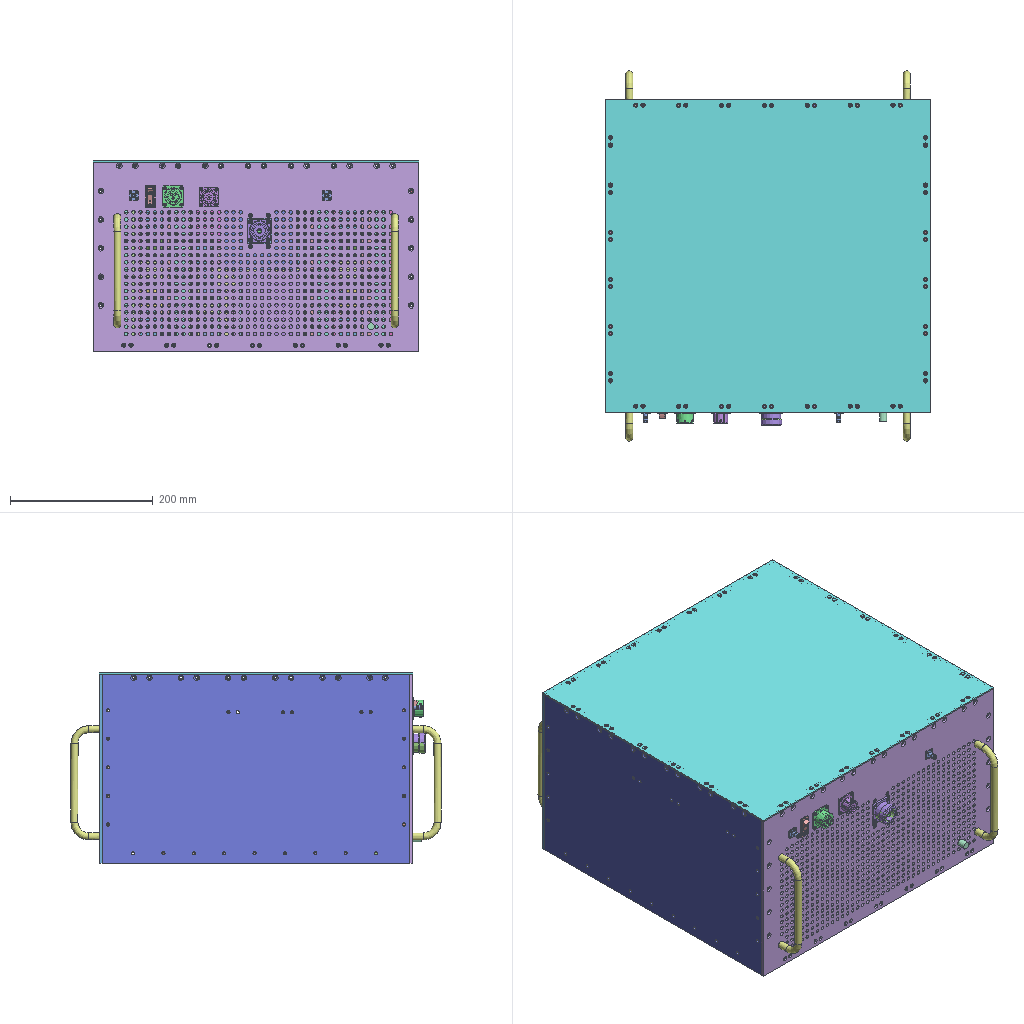Assembly | STEP file | 119 different items | 1042 placed | box 456 x 518 x 267 mm
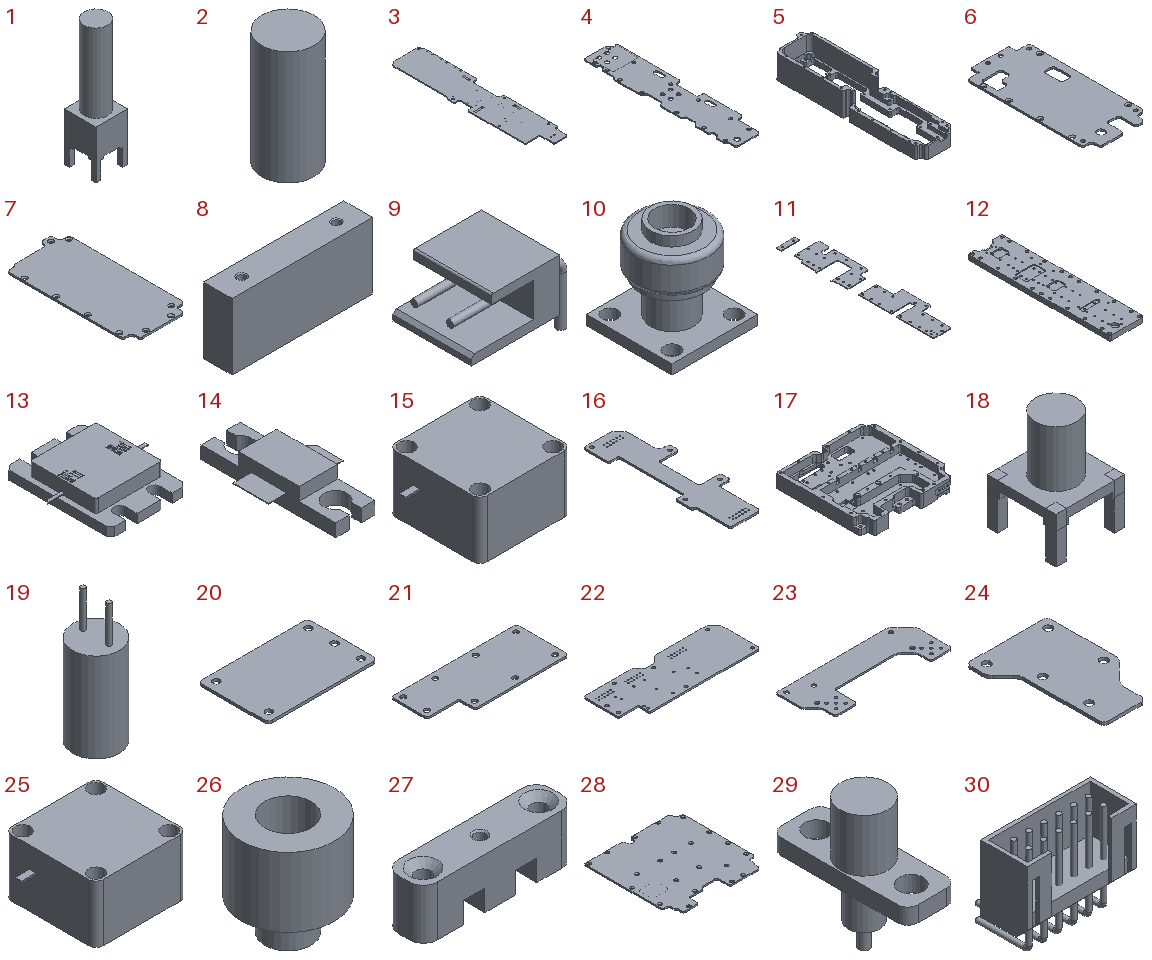Parts list (item | name | quantity | parent item | size | volume):
1 | MCX-KHD20 | x16 | in Final stage amplifier_MODEL | 6 x 6 x 24.3 mm | 456.556 mm3
2 | 1000uf-80V | x64 | in Final stage amplifier control, 48V power filter board_MODEL | 18 x 18 x 39 mm | 9924 mm3
3 | SOLID | x16 | in Final stage amplifier control | 40.98 x 193.1 x 1.2 mm | 8227 mm3
4 | Final stage amplifier cavity inner cover | x16 | in Final stage amplifier_MODEL | 41.47 x 194.01 x 1.5 mm | 9143 mm3
5 | Final stage amplifier cavity | x16 | in Final stage amplifier_MODEL | 49 x 204 x 32.1 mm | 62849 mm3
6 | Final stage amplifier cover 1 | x16 | in Final stage amplifier_MODEL | 49 x 104.5 x 1.5 mm | 6573 mm3
7 | Final stage cover 2 | x16 | in Final stage amplifier_MODEL | 49 x 105.5 x 1.5 mm | 7174 mm3
8 | Final stage amplifier press block | x16 | in Final stage amplifier_MODEL | 29.61 x 6 x 14 mm | 2437 mm3
9 | JL27-02ZJW | x16 | in Final stage amplifier_MODEL | 12.9 x 8.72 x 9.401 mm | 271.213 mm3
10 | N-KFD98 | x32 | in Final stage amplifier_MODEL | 17.5 x 17.5 x 25 mm | 2388 mm3
11 | Final stage amplifier 00 | x16 | in Final stage amplifier_MODEL | 34.739 x 191 x 0.832 mm | 3190 mm3
12 | 53005900 final-stage amplifier red copper | x16 | in Final stage amplifier_MODEL | 49 x 204 x 7 mm | 64981 mm3
13 | GN5359P300V40 | x16 | in Final stage amplifier_MODEL | 23 x 24.1 x 5 mm | 1437 mm3
14 | YP40601625T | x16 | in Final stage amplifier_MODEL | 11.3 x 20.43 x 3.88 mm | 294.314 mm3
15 | UIYDI1212B5300T5900 | x32 | in Final stage amplifier_MODEL | 16.7 x 12.7 x 8 mm | 1173 mm3
16 | 推动功放控制2PCB | x8 | in Driver amplifier module_MODEL | 29.18 x 90.51 x 1.2 mm | 1855 mm3
17 | Driver amplifier module cavity | x8 | in Driver amplifier module_MODEL | 99 x 98 x 14 mm | 63567 mm3
18 | MCX-JHD | x16 | in Driver amplifier module_MODEL | 6 x 6 x 8.9 mm | 97.715 mm3
19 | 118EC225 capacitor | x8 | in Driver amplifier module_MODEL | 6.3 x 6.3 x 17 mm | 376.897 mm3
20 | Driver amplifier PA2PCB | x8 | in Driver amplifier module_MODEL | 34 x 21.66 x 0.832 mm | 597.158 mm3
21 | Driver amplifier PA3PCB | x8 | in Driver amplifier module_MODEL | 52.1 x 21.66 x 0.832 mm | 840 mm3
22 | 推动功放控制1PCB | x8 | in Driver amplifier module_MODEL | 89.69 x 31.78 x 1.2 mm | 3157 mm3
23 | 推动功放1分2PCB | x8 | in Driver amplifier module_MODEL | 66.71 x 26.09 x 0.832 mm | 967.615 mm3
24 | Driver amplifier PA1PCB | x8 | in Driver amplifier module_MODEL | 21.48 x 32.08 x 0.832 mm | 418.678 mm3
25 | UIYDI1212B2800T3400 | x8 | in Driver amplifier module_MODEL | 16.7 x 12.7 x 8 mm | 1173 mm3
26 | Solder post | x32 | in Driver amplifier module_MODEL | 4 x 4 x 4.4 mm | 32.673 mm3
27 | Driver amplifier partition | x16 | in Driver amplifier module_MODEL | 21.48 x 5.5 x 7.1 mm | 643.148 mm3
28 | Driver amplifier module cover | x8 | in Driver amplifier module_MODEL | 99 x 98 x 1.5 mm | 12973 mm3
29 | MCX-KFD1 | x12 | in Driver amplifier module_MODEL, 1 to 8 power divider | 4.7 x 13 x 12.4 mm | 185.301 mm3
30 | JL24-12ZJW | x19 | in Driver amplifier module_MODEL, VSWR protection_MODEL, Control module_MODEL, Front stage module_MODEL | 14.6 x 9.1 x 12.075 mm | 379.843 mm3
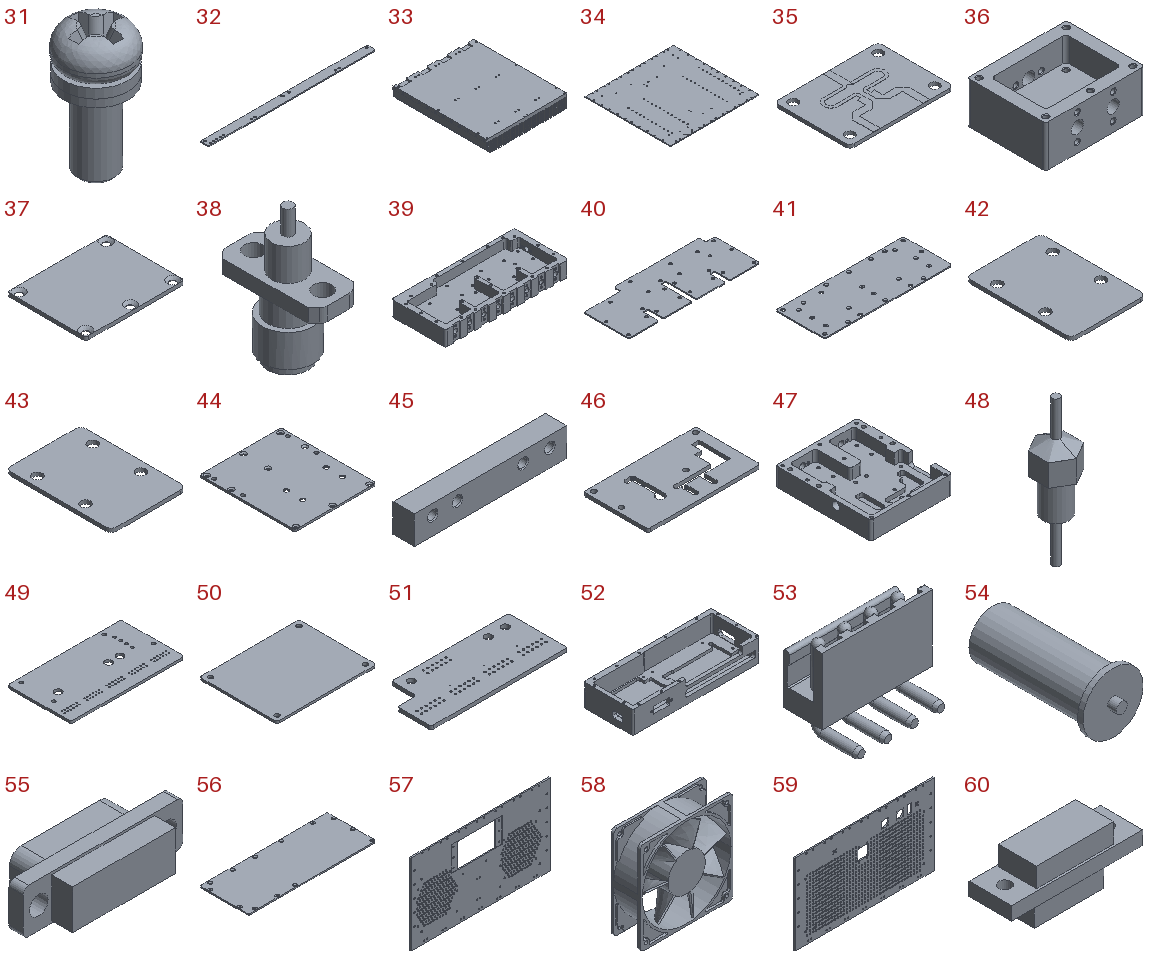31 | Pan head combination screw M2X5 | x8 | in Driver amplifier module_MODEL | 3.5 x 3.5 x 6.7 mm | 32.079 mm3
32 | Power supply board | x4 | in Heat sink | 198 x 10 x 1.2 mm | 2320 mm3
33 | SOLID | x4 | in Heat sink | 200 x 230 x 33.3 mm | 583013 mm3
34 | Chassis bottom plate | x1 | in 27003500整机机箱 | 450 x 430 x 4 mm | 764514 mm3
35 | 1 to 2 power divider PCB | x1 | in 1 to 2 power divider | 25 x 18.18 x 0.832 mm | 351.83 mm3
36 | 1 to 2 power divider cavity | x1 | in 1 to 2 power divider | 33.2 x 26.38 x 14 mm | 8149 mm3
37 | 1 to 2 power divider cover | x1 | in 1 to 2 power divider | 33.2 x 26.38 x 1.2 mm | 1010 mm3
38 | SMA-KFD-4-3 | x14 | in 1 to 2 power divider, 1 to 8 power divider, VSWR protection_MODEL, Frequency synthesizer_MODEL, Front stage module_MODEL | 6.28 x 12.6 x 16.5 mm | 359.204 mm3
39 | 1 to 8 power divider cavity | x1 | in 1 to 8 power divider | 120.8 x 52.94 x 15 mm | 53441 mm3
40 | 1 to 8 power divider PCB | x1 | in 1 to 8 power divider | 110 x 43.34 x 0.832 mm | 3538 mm3
41 | 1 to 8 power divider cover | x1 | in 1 to 8 power divider | 141.709 x 54.52 x 1.2 mm | 9052 mm3
42 | VSWR protection V+PCB | x1 | in VSWR protection_MODEL | 17.08 x 24.07 x 0.832 mm | 328.245 mm3
43 | VSWR protection V-PCB | x1 | in VSWR protection_MODEL | 17.08 x 24.07 x 0.832 mm | 328.245 mm3
44 | VSWR protection cover | x1 | in VSWR protection_MODEL | 60 x 70.12 x 1.5 mm | 6124 mm3
45 | VSWR protection spacer strip | x1 | in VSWR protection_MODEL | 43.08 x 5.97 x 8 mm | 1913 mm3
46 | VSWR protection control PCB | x1 | in VSWR protection_MODEL | 51.4 x 29.58 x 1.6 mm | 2088 mm3
47 | VSWR protection cavity | x1 | in VSWR protection_MODEL | 60 x 70.12 x 13.5 mm | 30547 mm3
48 | Feed through capacitor M3 | x4 | in VSWR protection_MODEL | 4 x 4.619 x 16.5 mm | 73.685 mm3
49 | Control module PCB | x1 | in Control module_MODEL | 76.14 x 42.52 x 1.6 mm | 5007 mm3
50 | Control module MCU PCB | x1 | in Control module_MODEL | 54.57 x 42.52 x 1.2 mm | 2759 mm3
51 | Control module adapter PCB | x1 | in Control module_MODEL | 60.512 x 26.172 x 1.6 mm | 2296 mm3
52 | Control module cavity | x1 | in Control module_MODEL | 141.709 x 54.52 x 25 mm | 59399 mm3
53 | JL27-04ZJW | x1 | in Control module_MODEL | 16.44 x 9.4 x 13.15 mm | 524.314 mm3
54 | Copper solder post M3-11-4.4 | x17 | in Control module_MODEL, 220V main power merge board_MODEL, 48V power filter board_MODEL, 24V input power board_MODEL | 5.5 x 11.8 x 5.5 mm | 131.403 mm3
55 | J30J-21TK | x1 | in Control module_MODEL | 27.4 x 10.9 x 7.6 mm | 1017 mm3
56 | Control module cover | x1 | in Control module_MODEL | 141.709 x 54.52 x 1.5 mm | 11459 mm3
57 | Chassis front panel | x1 | in 27003500整机机箱 | 456 x 4 x 264.7 mm | 404809 mm3
58 | Fan 9WV1224P1H00100 | x2 | in 27003500整机机箱 | 120 x 39.419 x 120 mm | 145446 mm3
59 | Main chassis rear panel | x1 | in 27003500整机机箱 | 456 x 4 x 264.7 mm | 416377 mm3
60 | J30J-15ZKP | x1 | in Frequency synthesizer_MODEL | 23.5 x 7.6 x 10.5 mm | 877.754 mm3
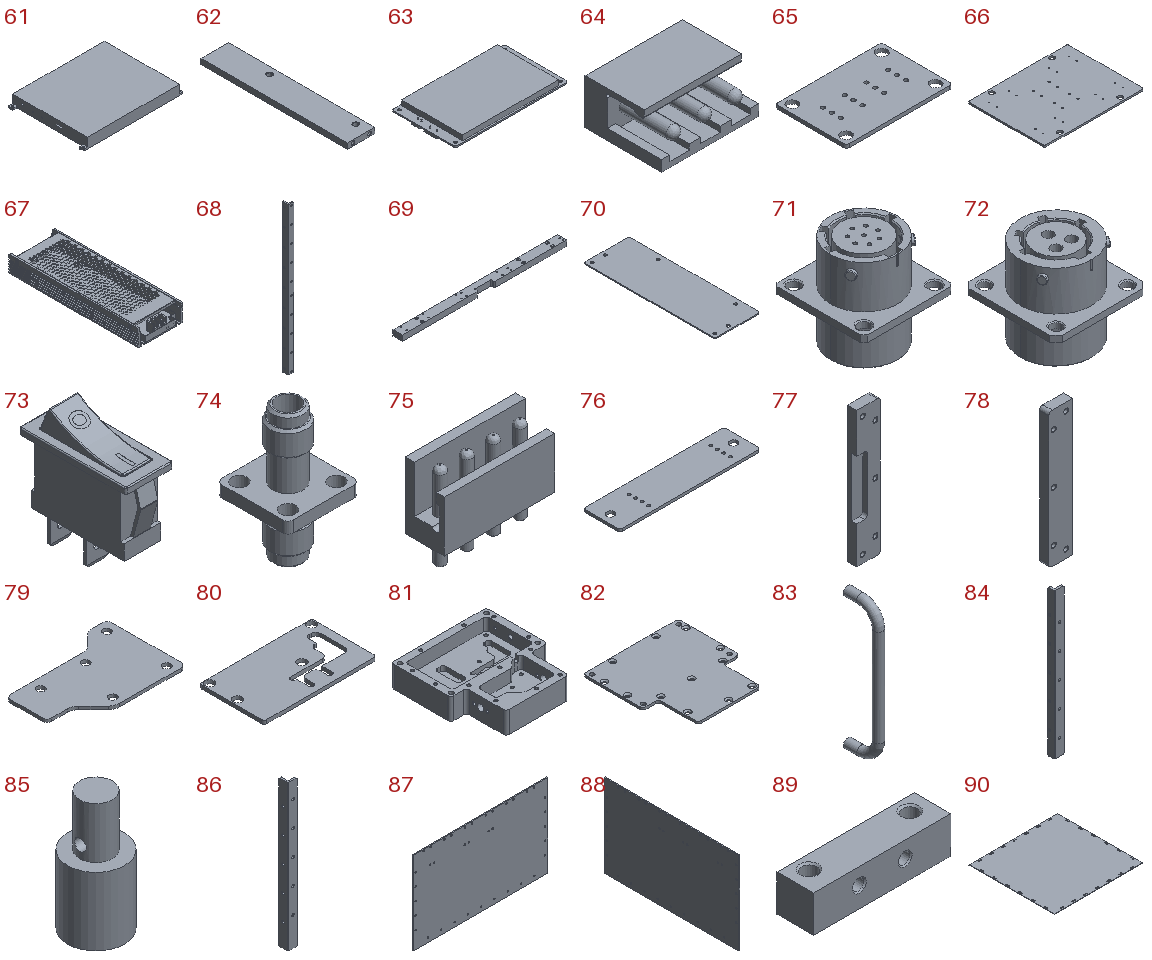61 | SOLID | x1 | in Frequency synthesizer_MODEL | 200 x 150 x 20 mm | 552493 mm3
62 | Power mounting plate | x2 | in 27003500整机机箱 | 20 x 107 x 4 mm | 8429 mm3
63 | Screen OCM800480T500 | x1 | in 27003500整机机箱 | 143.47 x 81 x 10.1 mm | 81087 mm3
64 | JL27-03ZJB | x4 | in 220V main power merge board_MODEL | 12.48 x 11.4 x 5.8 mm | 382.21 mm3
65 | SOLID | x1 | in 220V main power merge board_MODEL | 47.38 x 31.85 x 1.6 mm | 2258 mm3
66 | SOLID | x2 | in 48V power filter board_MODEL | 96.757 x 74.5 x 1.6 mm | 11377 mm3
67 | Power module UHP-500(R) | x1 | in 27003500整机机箱 | 81 x 232 x 31 mm | 117475 mm3
68 | L shaped aluminium angle 1 | x2 | in 27003500整机机箱 | 13 x 15 x 359 mm | 26222 mm3
69 | Chassis spacer strip | x2 | in 27003500整机机箱 | 450 x 25 x 15 mm | 159345 mm3
70 | Mounting block | x1 | in 27003500整机机箱 | 55 x 160 x 1.2 mm | 10487 mm3
71 | Connector Y50X5-1208Z30K | x1 | in 27003500整机机箱 | 27 x 27 x 29.03 mm | 7701 mm3
72 | Connector Y50DX5-1403Z30K | x1 | in 27003500整机机箱 | 30 x 30 x 29.03 mm | 10352 mm3
73 | Rocker switch KCD3-50A | x1 | in 27003500整机机箱 | 13.7 x 31 x 35.877 mm | 6384 mm3
74 | Connector SMA-KKF | x2 | in 27003500整机机箱 | 12.7 x 12.7 x 23.5 mm | 626.237 mm3
75 | JL27-04ZJB | x2 | in 24V input power board_MODEL | 16.44 x 5.8 x 13.5 mm | 568.163 mm3
76 | SOLID | x1 | in 24V input power board_MODEL | 85 x 22 x 1.6 mm | 2905 mm3
77 | Screen mounting block 1 | x1 | in 27003500整机机箱 | 14.18 x 5.5 x 81 mm | 5488 mm3
78 | Screen mounting block 2 | x1 | in 27003500整机机箱 | 14.19 x 5.5 x 81 mm | 6175 mm3
79 | Front stage RF PCB | x1 | in Front stage module_MODEL | 32.08 x 21.48 x 0.832 mm | 418.678 mm3
80 | Front stage control PCB | x1 | in Front stage module_MODEL | 51.4 x 29.58 x 1.6 mm | 2071 mm3
81 | Front stage cavity | x1 | in Front stage module_MODEL | 61.4 x 64.23 x 14 mm | 29019 mm3
82 | Front stage cover | x1 | in Front stage module_MODEL | 61.4 x 64.23 x 1.5 mm | 4977 mm3
83 | SOLID | x8 | in 把手10X150X40-M5 | 10 x 40 x 160 mm | 15544 mm3
84 | L shaped aluminium angle 2 | x1 | in 27003500整机机箱 | 15 x 10.7 x 233 mm | 15474 mm3
85 | Ground post | x1 | in 27003500整机机箱 | 10 x 10 x 21 mm | 1161 mm3
86 | SOLID | x6 | in L shaped aluminium angle 3 | 15 x 15 x 233 mm | 18483 mm3
87 | Chassis left side panel | x1 | in 27003500整机机箱 | 430 x 3 x 264.7 mm | 339377 mm3
88 | Chassis right side panel | x1 | in 27003500整机机箱 | 3 x 430 x 264.7 mm | 339377 mm3
89 | Connector mounting block | x39 | in 27003500整机机箱 | 30 x 8 x 8 mm | 1701 mm3
90 | Chassis cover | x1 | in 27003500整机机箱 | 456 x 438 x 2 mm | 397913 mm3
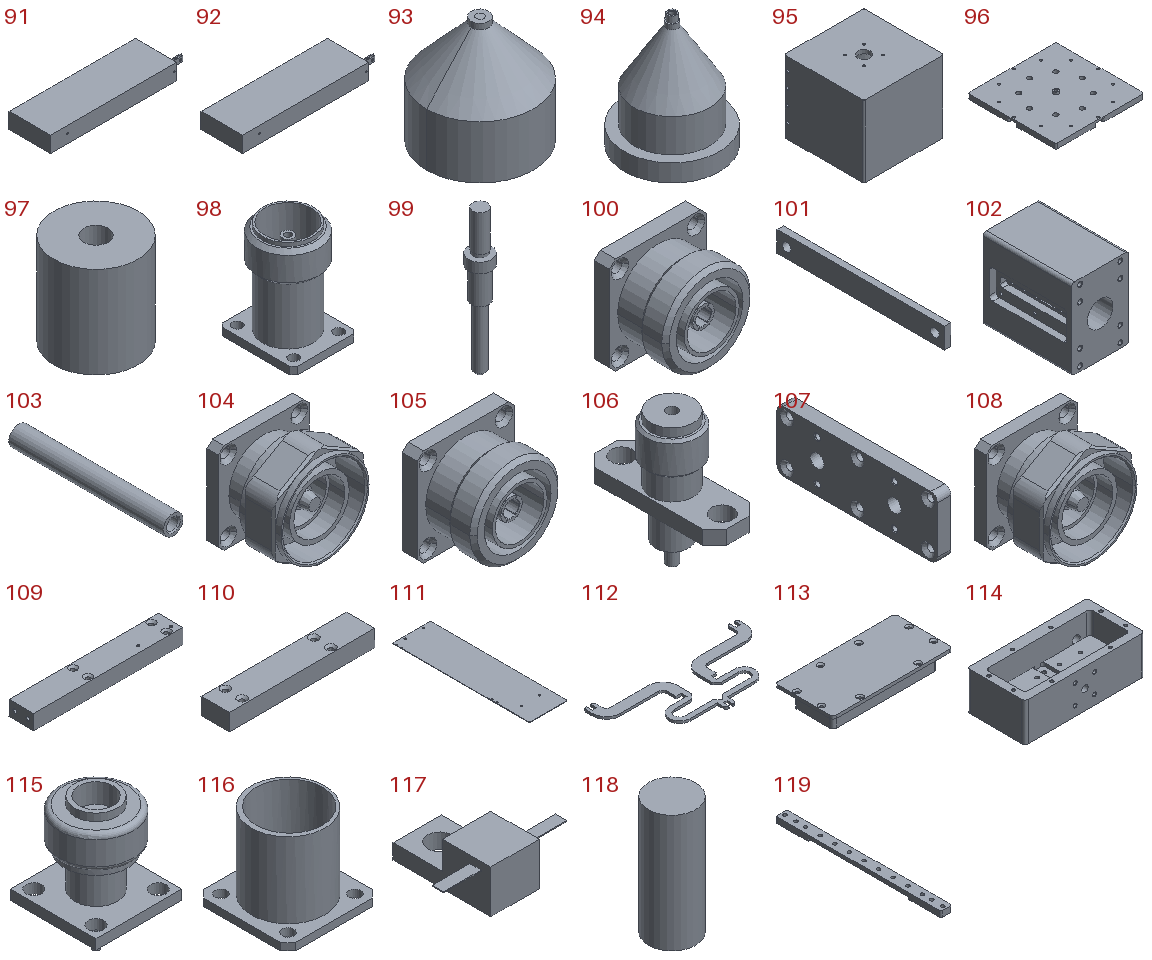91 | COMPOUND | x2 | in Power module UHP-3200 | 363.8 x 107 x 41 mm | 1432156 mm3
92 | COMPOUND | x2 | in Power module UHP-3200 | 363.8 x 107 x 41 mm | 1432156 mm3
93 | LPFD27003500MHz_step | x1 | in 8-in-1 radial waveguide | 96.34 x 96.34 x 102.43 mm | 664889 mm3
94 | Radial combiner inner cavity | x1 | in 8-in-1 radial waveguide | 76 x 76 x 96.43 mm | 185605 mm3
95 | Radial combiner outer cavity | x1 | in 8-in-1 radial waveguide | 107 x 107 x 96.43 mm | 625151 mm3
96 | Combiner cover | x1 | in 8-in-1 radial waveguide | 107 x 107 x 9 mm | 64733 mm3
97 | Radial combiner dielectric | x8 | in 8-in-1 radial waveguide | 5.5 x 5.5 x 6 mm | 130.486 mm3
98 | Connector N-KFD612 | x8 | in 8-in-1 radial waveguide | 17 x 20 x 26.6 mm | 3584 mm3
99 | Radial combiner probe | x8 | in 8-in-1 radial waveguide | 3.2 x 3.2 x 19.92 mm | 64.491 mm3
100 | 连接器 L29-KFD-9 | x2 | in 8-in-1 radial waveguide, Coupler_MODEL | 32 x 30.7 x 32 mm | 11064 mm3
101 | Coupler coupling plate | x2 | in Coupler_MODEL | 1 x 26 x 3.21 mm | 80.805 mm3
102 | Coupler cavity | x1 | in Coupler_MODEL | 35.5 x 55 x 50 mm | 76376 mm3
103 | Coupler copper rod | x1 | in Coupler_MODEL | 7 x 55 x 7 mm | 1826 mm3
104 | Connector L29-50JFDA | x1 | in Coupler_MODEL | 32 x 30.6 x 35.094 mm | 12023 mm3
105 | Connector L29-50KFDA | x1 | in Coupler_MODEL | 32 x 27.7 x 32 mm | 10941 mm3
106 | Connector SMA-KFD561 | x4 | in Coupler_MODEL | 6.3 x 16 x 16 mm | 381.279 mm3
107 | Coupler cover | x2 | in Coupler_MODEL | 4 x 47.8 x 18 mm | 3182 mm3
108 | Connector L29-JFD | x1 | in Coupler_MODEL | 32 x 30.6 x 35.094 mm | 12630 mm3
109 | Chassis spacer strip 1 | x1 | in 27003500整机机箱 | 150 x 25 x 15 mm | 54927 mm3
110 | Chassis spacer strip 2 | x1 | in 27003500整机机箱 | 130 x 25 x 15 mm | 47613 mm3
111 | Combiner mounting plate | x1 | in 27003500整机机箱 | 90 x 325.8 x 1 mm | 29233 mm3
112 | 2-in-1 splitter plate | x8 | in 2-in-1 combiner | 53.51 x 24.649 x 0.8 mm | 239.301 mm3
113 | 2-in-1 cover | x8 | in 2-in-1 combiner | 78 x 37.65 x 12.6 mm | 23932 mm3
114 | 2-in-1 cavity | x8 | in 2-in-1 combiner | 78 x 37.65 x 25 mm | 47258 mm3
115 | N-KFD1005NT | x8 | in 2-in-1 combiner | 17.5 x 17.5 x 27 mm | 2315 mm3
116 | SOLID | x32 | in N-JFD7 | 25 x 25 x 32 mm | 2535 mm3
117 | RHD-50W | x8 | in 2-in-1 combiner | 16.4 x 13 x 5.7 mm | 303.667 mm3
118 | SOLID | x256 | in PTFE pad | 2 x 2 x 5 mm | 15.708 mm3
119 | SOLID | x4 | in Combiner mounting block | 15 x 226 x 8 mm | 19553 mm3
Placements (level | parent | child | x y z in mm | rotation matrix by rows), first 275 of 1265 lines:
1 | 27003500整机机箱 | Power amplifier module | -114.646 -154.887 86.101 | 0 0 -1 0 1 0 1 0 0
2 | Power amplifier module | Final stage amplifier_MODEL | -3.876 14.0 2.0 | 1 0 0 0 1 0 0 0 1
3 | Final stage amplifier_MODEL | MCX-KHD20 | 65.091 -16.608 213.097 | 0.7071 -0.7071 0 0.7071 0.7071 0 0 0 1
3 | Final stage amplifier_MODEL | Final stage amplifier control | -1016.416 -878.875 183.732 | 1 0 0 0 1 0 0 0 1
4 | Final stage amplifier control | 1000uf-80V | 1043.852 1010.557 9.0 | 0 0 -1 0 1 0 1 0 -0
4 | Final stage amplifier control | 1000uf-80V | 1043.852 1028.557 9.0 | 0 0 -1 0 1 0 1 0 0
4 | Final stage amplifier control | 1000uf-80V | 1043.852 1046.557 9.0 | 0 0 -1 0 1 0 1 0 0
4 | Final stage amplifier control | SOLID | 0.0 0.0 0.0 | 1 0 0 0 1 0 0 0 1
3 | Final stage amplifier_MODEL | Final stage amplifier cavity inner cover | -691.532 -865.508 179.032 | 1 0 0 0 1 0 0 0 1
3 | Final stage amplifier_MODEL | Final stage amplifier cavity | 0.0 0.0 0.0 | 1 0 0 0 1 0 0 0 1
3 | Final stage amplifier_MODEL | Final stage amplifier cover 1 | 0.0 -0.0 1.6 | 1 0 0 0 1 0 0 0 1
3 | Final stage amplifier_MODEL | Final stage cover 2 | 0.0 0.0 2.6 | 1 0 0 0 1 0 0 0 1
3 | Final stage amplifier_MODEL | Final stage amplifier press block | 0.0 0.0 0.068 | 1 0 0 0 1 0 0 0 1
3 | Final stage amplifier_MODEL | JL27-02ZJW | 12.636 -4.01 186.632 | 0 -1 0 1 0 0 0 0 1
3 | Final stage amplifier_MODEL | N-KFD98 | 4.016 185.25 171.564 | 0 -1 0 0 0 1 -1 0 0
3 | Final stage amplifier_MODEL | Final stage amplifier 00 | -632.632 -865.508 171.364 | 1 0 0 0 1 0 0 0 1
3 | Final stage amplifier_MODEL | 53005900 final-stage amplifier red copper | 0.0 0.0 170.532 | 1 0 0 0 1 0 0 0 1
3 | Final stage amplifier_MODEL | GN5359P300V40 | 3.816 122.165 169.132 | 0 -1 0 1 0 0 0 0 1
3 | Final stage amplifier_MODEL | YP40601625T | 5.598 38.846 169.532 | 0 -1 0 1 0 0 0 0 1
3 | Final stage amplifier_MODEL | UIYDI1212B5300T5900 | 6.466 168.94 176.632 | 0 -1 0 -1 0 0 0 0 -1
3 | Final stage amplifier_MODEL | UIYDI1212B5300T5900 | 6.466 88.08 176.632 | 0 -1 0 -1 0 0 0 0 -1
3 | Final stage amplifier_MODEL | N-KFD98 | 4.016 185.25 171.564 | 0 -1 0 0 0 1 -1 0 0
2 | Power amplifier module | Driver amplifier module_MODEL | -904.308 -851.508 197.464 | 1 0 0 0 1 0 0 0 1
3 | Driver amplifier module_MODEL | 推动功放控制2PCB | -0.0 0.0 -3.832 | 1 0 0 0 1 0 0 0 1
3 | Driver amplifier module_MODEL | Driver amplifier module cavity | -0.0 0.0 -0.832 | 1 0 0 0 1 0 0 0 1
3 | Driver amplifier module_MODEL | MCX-JHD | 899.678 861.268 -2.132 | 1 0 0 0 -1 0 0 0 -1
3 | Driver amplifier module_MODEL | 118EC225 capacitor | 888.644 0.2536 866.668 | 0 0 1 0 1 0 -1 0 0
3 | Driver amplifier module_MODEL | Driver amplifier PA2PCB | 0.0 0.0 0.0 | 1 0 0 0 1 0 0 0 1
3 | Driver amplifier module_MODEL | Driver amplifier PA3PCB | 0.0 0.0 0.0 | 1 0 0 0 1 0 0 0 1
3 | Driver amplifier module_MODEL | 推动功放控制1PCB | 0.0 0.0 0.368 | 1 0 0 0 1 0 0 0 1
3 | Driver amplifier module_MODEL | 推动功放1分2PCB | 0.0 0.0 0.0 | 1 0 0 0 1 0 0 0 1
3 | Driver amplifier module_MODEL | Driver amplifier PA1PCB | 0.0 0.0 0.0 | 1 0 0 0 1 0 0 0 1
3 | Driver amplifier module_MODEL | MCX-JHD | 949.678 861.268 -2.132 | 1 0 0 0 -1 0 0 0 -1
3 | Driver amplifier module_MODEL | UIYDI1212B2800T3400 | 896.718 888.488 5.268 | 0 1 0 1 0 0 0 0 -1
3 | Driver amplifier module_MODEL | Solder post | 905.16 943.44 -3.832 | 1 0 0 0 1 0 0 0 1
3 | Driver amplifier module_MODEL | Driver amplifier partition | 0.0 0.0 0.0 | 1 0 0 0 1 0 0 0 1
3 | Driver amplifier module_MODEL | Driver amplifier partition | 1824.776 -66.95 0.0 | 0 -1 0 1 0 0 0 0 1
3 | Driver amplifier module_MODEL | Driver amplifier module cover | 0.0 0.0 0.0 | 1 0 0 0 1 0 0 0 1
3 | Driver amplifier module_MODEL | MCX-KFD1 | 965.238 852.098 0.6 | 0 -1 0 0 0 -1 1 0 -0
3 | Driver amplifier module_MODEL | Solder post | 906.19 885.113 -3.832 | 1 0 0 0 1 0 0 0 1
3 | Driver amplifier module_MODEL | Solder post | 928.208 917.018 -3.832 | 1 0 0 0 1 0 0 0 1
3 | Driver amplifier module_MODEL | Solder post | 928.208 885.113 -3.832 | 1 0 0 0 1 0 0 0 1
3 | Driver amplifier module_MODEL | JL24-12ZJW | 915.278 858.078 -0.732 | -1 0 0 0 0 -1 0 -1 0
3 | Driver amplifier module_MODEL | Pan head combination screw M2X5 | 891.618 893.588 1.168 | 1 0 0 0 1 0 0 0 1
2 | Power amplifier module | Heat sink | 0.0 10.0 0.0 | 1 0 0 0 1 0 0 0 1
3 | Heat sink | Power supply board | -73.325 -121.393 166.732 | 1 0 0 0 1 0 0 0 1
3 | Heat sink | SOLID | 0.0 0.0 0.0 | 1 0 0 0 1 0 0 0 1
2 | Power amplifier module | Final stage amplifier_MODEL | 46.124 14.0 2.0 | 1 0 0 0 1 0 0 0 1
3 | Final stage amplifier_MODEL | MCX-KHD20 | 65.091 -16.608 213.097 | 0.7071 -0.7071 0 0.7071 0.7071 0 0 0 1
3 | Final stage amplifier_MODEL | Final stage amplifier control | -1016.416 -878.875 183.732 | 1 0 0 0 1 0 0 0 1
4 | Final stage amplifier control | 1000uf-80V | 1043.852 1010.557 9.0 | 0 0 -1 0 1 0 1 0 -0
4 | Final stage amplifier control | 1000uf-80V | 1043.852 1028.557 9.0 | 0 0 -1 0 1 0 1 0 0
4 | Final stage amplifier control | 1000uf-80V | 1043.852 1046.557 9.0 | 0 0 -1 0 1 0 1 0 0
4 | Final stage amplifier control | SOLID | 0.0 0.0 0.0 | 1 0 0 0 1 0 0 0 1
3 | Final stage amplifier_MODEL | Final stage amplifier cavity inner cover | -691.532 -865.508 179.032 | 1 0 0 0 1 0 0 0 1
3 | Final stage amplifier_MODEL | Final stage amplifier cavity | 0.0 0.0 0.0 | 1 0 0 0 1 0 0 0 1
3 | Final stage amplifier_MODEL | Final stage amplifier cover 1 | 0.0 -0.0 1.6 | 1 0 0 0 1 0 0 0 1
3 | Final stage amplifier_MODEL | Final stage cover 2 | 0.0 0.0 2.6 | 1 0 0 0 1 0 0 0 1
3 | Final stage amplifier_MODEL | Final stage amplifier press block | 0.0 0.0 0.068 | 1 0 0 0 1 0 0 0 1
3 | Final stage amplifier_MODEL | JL27-02ZJW | 12.636 -4.01 186.632 | 0 -1 0 1 0 0 0 0 1
3 | Final stage amplifier_MODEL | N-KFD98 | 4.016 185.25 171.564 | 0 -1 0 0 0 1 -1 0 0
3 | Final stage amplifier_MODEL | Final stage amplifier 00 | -632.632 -865.508 171.364 | 1 0 0 0 1 0 0 0 1
3 | Final stage amplifier_MODEL | 53005900 final-stage amplifier red copper | 0.0 0.0 170.532 | 1 0 0 0 1 0 0 0 1
3 | Final stage amplifier_MODEL | GN5359P300V40 | 3.816 122.165 169.132 | 0 -1 0 1 0 0 0 0 1
3 | Final stage amplifier_MODEL | YP40601625T | 5.598 38.846 169.532 | 0 -1 0 1 0 0 0 0 1
3 | Final stage amplifier_MODEL | UIYDI1212B5300T5900 | 6.466 168.94 176.632 | 0 -1 0 -1 0 0 0 0 -1
3 | Final stage amplifier_MODEL | UIYDI1212B5300T5900 | 6.466 88.08 176.632 | 0 -1 0 -1 0 0 0 0 -1
3 | Final stage amplifier_MODEL | N-KFD98 | 4.016 185.25 171.564 | 0 -1 0 0 0 1 -1 0 0
2 | Power amplifier module | Final stage amplifier_MODEL | 96.124 14.0 2.0 | 1 0 0 0 1 0 0 0 1
3 | Final stage amplifier_MODEL | MCX-KHD20 | 65.091 -16.608 213.097 | 0.7071 -0.7071 0 0.7071 0.7071 0 0 0 1
3 | Final stage amplifier_MODEL | Final stage amplifier control | -1016.416 -878.875 183.732 | 1 0 0 0 1 0 0 0 1
4 | Final stage amplifier control | 1000uf-80V | 1043.852 1010.557 9.0 | 0 0 -1 0 1 0 1 0 -0
4 | Final stage amplifier control | 1000uf-80V | 1043.852 1028.557 9.0 | 0 0 -1 0 1 0 1 0 0
4 | Final stage amplifier control | 1000uf-80V | 1043.852 1046.557 9.0 | 0 0 -1 0 1 0 1 0 0
4 | Final stage amplifier control | SOLID | 0.0 0.0 0.0 | 1 0 0 0 1 0 0 0 1
3 | Final stage amplifier_MODEL | Final stage amplifier cavity inner cover | -691.532 -865.508 179.032 | 1 0 0 0 1 0 0 0 1
3 | Final stage amplifier_MODEL | Final stage amplifier cavity | 0.0 0.0 0.0 | 1 0 0 0 1 0 0 0 1
3 | Final stage amplifier_MODEL | Final stage amplifier cover 1 | 0.0 -0.0 1.6 | 1 0 0 0 1 0 0 0 1
3 | Final stage amplifier_MODEL | Final stage cover 2 | 0.0 0.0 2.6 | 1 0 0 0 1 0 0 0 1
3 | Final stage amplifier_MODEL | Final stage amplifier press block | 0.0 0.0 0.068 | 1 0 0 0 1 0 0 0 1
3 | Final stage amplifier_MODEL | JL27-02ZJW | 12.636 -4.01 186.632 | 0 -1 0 1 0 0 0 0 1
3 | Final stage amplifier_MODEL | N-KFD98 | 4.016 185.25 171.564 | 0 -1 0 0 0 1 -1 0 0
3 | Final stage amplifier_MODEL | Final stage amplifier 00 | -632.632 -865.508 171.364 | 1 0 0 0 1 0 0 0 1
3 | Final stage amplifier_MODEL | 53005900 final-stage amplifier red copper | 0.0 0.0 170.532 | 1 0 0 0 1 0 0 0 1
3 | Final stage amplifier_MODEL | GN5359P300V40 | 3.816 122.165 169.132 | 0 -1 0 1 0 0 0 0 1
3 | Final stage amplifier_MODEL | YP40601625T | 5.598 38.846 169.532 | 0 -1 0 1 0 0 0 0 1
3 | Final stage amplifier_MODEL | UIYDI1212B5300T5900 | 6.466 168.94 176.632 | 0 -1 0 -1 0 0 0 0 -1
3 | Final stage amplifier_MODEL | UIYDI1212B5300T5900 | 6.466 88.08 176.632 | 0 -1 0 -1 0 0 0 0 -1
3 | Final stage amplifier_MODEL | N-KFD98 | 4.016 185.25 171.564 | 0 -1 0 0 0 1 -1 0 0
2 | Power amplifier module | Final stage amplifier_MODEL | 146.125 14.0 2.0 | 1 0 0 0 1 0 0 0 1
3 | Final stage amplifier_MODEL | MCX-KHD20 | 65.091 -16.608 213.097 | 0.7071 -0.7071 0 0.7071 0.7071 0 0 0 1
3 | Final stage amplifier_MODEL | Final stage amplifier control | -1016.416 -878.875 183.732 | 1 0 0 0 1 0 0 0 1
4 | Final stage amplifier control | 1000uf-80V | 1043.852 1010.557 9.0 | 0 0 -1 0 1 0 1 0 -0
4 | Final stage amplifier control | 1000uf-80V | 1043.852 1028.557 9.0 | 0 0 -1 0 1 0 1 0 0
4 | Final stage amplifier control | 1000uf-80V | 1043.852 1046.557 9.0 | 0 0 -1 0 1 0 1 0 0
4 | Final stage amplifier control | SOLID | 0.0 0.0 0.0 | 1 0 0 0 1 0 0 0 1
3 | Final stage amplifier_MODEL | Final stage amplifier cavity inner cover | -691.532 -865.508 179.032 | 1 0 0 0 1 0 0 0 1
3 | Final stage amplifier_MODEL | Final stage amplifier cavity | 0.0 0.0 0.0 | 1 0 0 0 1 0 0 0 1
3 | Final stage amplifier_MODEL | Final stage amplifier cover 1 | 0.0 -0.0 1.6 | 1 0 0 0 1 0 0 0 1
3 | Final stage amplifier_MODEL | Final stage cover 2 | 0.0 0.0 2.6 | 1 0 0 0 1 0 0 0 1
3 | Final stage amplifier_MODEL | Final stage amplifier press block | 0.0 0.0 0.068 | 1 0 0 0 1 0 0 0 1
3 | Final stage amplifier_MODEL | JL27-02ZJW | 12.636 -4.01 186.632 | 0 -1 0 1 0 0 0 0 1
3 | Final stage amplifier_MODEL | N-KFD98 | 4.016 185.25 171.564 | 0 -1 0 0 0 1 -1 0 0
3 | Final stage amplifier_MODEL | Final stage amplifier 00 | -632.632 -865.508 171.364 | 1 0 0 0 1 0 0 0 1
3 | Final stage amplifier_MODEL | 53005900 final-stage amplifier red copper | 0.0 0.0 170.532 | 1 0 0 0 1 0 0 0 1
3 | Final stage amplifier_MODEL | GN5359P300V40 | 3.816 122.165 169.132 | 0 -1 0 1 0 0 0 0 1
3 | Final stage amplifier_MODEL | YP40601625T | 5.598 38.846 169.532 | 0 -1 0 1 0 0 0 0 1
3 | Final stage amplifier_MODEL | UIYDI1212B5300T5900 | 6.466 168.94 176.632 | 0 -1 0 -1 0 0 0 0 -1
3 | Final stage amplifier_MODEL | UIYDI1212B5300T5900 | 6.466 88.08 176.632 | 0 -1 0 -1 0 0 0 0 -1
3 | Final stage amplifier_MODEL | N-KFD98 | 4.016 185.25 171.564 | 0 -1 0 0 0 1 -1 0 0
2 | Power amplifier module | Driver amplifier module_MODEL | -804.308 -851.508 197.464 | 1 0 0 0 1 0 0 0 1
3 | Driver amplifier module_MODEL | 推动功放控制2PCB | -0.0 0.0 -3.832 | 1 0 0 0 1 0 0 0 1
3 | Driver amplifier module_MODEL | Driver amplifier module cavity | -0.0 0.0 -0.832 | 1 0 0 0 1 0 0 0 1
3 | Driver amplifier module_MODEL | MCX-JHD | 899.678 861.268 -2.132 | 1 0 0 0 -1 0 0 0 -1
3 | Driver amplifier module_MODEL | 118EC225 capacitor | 888.644 0.2536 866.668 | 0 0 1 0 1 0 -1 0 0
3 | Driver amplifier module_MODEL | Driver amplifier PA2PCB | 0.0 0.0 0.0 | 1 0 0 0 1 0 0 0 1
3 | Driver amplifier module_MODEL | Driver amplifier PA3PCB | 0.0 0.0 0.0 | 1 0 0 0 1 0 0 0 1
3 | Driver amplifier module_MODEL | 推动功放控制1PCB | 0.0 0.0 0.368 | 1 0 0 0 1 0 0 0 1
3 | Driver amplifier module_MODEL | 推动功放1分2PCB | 0.0 0.0 0.0 | 1 0 0 0 1 0 0 0 1
3 | Driver amplifier module_MODEL | Driver amplifier PA1PCB | 0.0 0.0 0.0 | 1 0 0 0 1 0 0 0 1
3 | Driver amplifier module_MODEL | MCX-JHD | 949.678 861.268 -2.132 | 1 0 0 0 -1 0 0 0 -1
3 | Driver amplifier module_MODEL | UIYDI1212B2800T3400 | 896.718 888.488 5.268 | 0 1 0 1 0 0 0 0 -1
3 | Driver amplifier module_MODEL | Solder post | 905.16 943.44 -3.832 | 1 0 0 0 1 0 0 0 1
3 | Driver amplifier module_MODEL | Driver amplifier partition | 0.0 0.0 0.0 | 1 0 0 0 1 0 0 0 1
3 | Driver amplifier module_MODEL | Driver amplifier partition | 1824.776 -66.95 0.0 | 0 -1 0 1 0 0 0 0 1
3 | Driver amplifier module_MODEL | Driver amplifier module cover | 0.0 0.0 0.0 | 1 0 0 0 1 0 0 0 1
3 | Driver amplifier module_MODEL | MCX-KFD1 | 965.238 852.098 0.6 | 0 -1 0 0 0 -1 1 0 -0
3 | Driver amplifier module_MODEL | Solder post | 906.19 885.113 -3.832 | 1 0 0 0 1 0 0 0 1
3 | Driver amplifier module_MODEL | Solder post | 928.208 917.018 -3.832 | 1 0 0 0 1 0 0 0 1
3 | Driver amplifier module_MODEL | Solder post | 928.208 885.113 -3.832 | 1 0 0 0 1 0 0 0 1
3 | Driver amplifier module_MODEL | JL24-12ZJW | 915.278 858.078 -0.732 | -1 0 0 0 0 -1 0 -1 0
3 | Driver amplifier module_MODEL | Pan head combination screw M2X5 | 891.618 893.588 1.168 | 1 0 0 0 1 0 0 0 1
1 | 27003500整机机箱 | Chassis bottom plate | -110.778 0.4935 59.877 | 1 0 0 0 1 0 0 0 1
1 | 27003500整机机箱 | 1 to 2 power divider | -151.569 153.008 213.397 | 1 0 0 0 1 0 0 0 1
2 | 1 to 2 power divider | 1 to 2 power divider PCB | -252.164 -254.35 87.277 | 1 0 0 0 1 0 0 0 1
2 | 1 to 2 power divider | 1 to 2 power divider cavity | 0.0 0.0 0.0 | 1 0 0 0 1 0 0 0 1
2 | 1 to 2 power divider | 1 to 2 power divider cover | 0.0 0.0 0.0 | 1 0 0 0 1 0 0 0 1
2 | 1 to 2 power divider | SMA-KFD-4-3 | -149.548 -150.773 88.047 | 0 1 0 0 0 -1 -1 0 0
2 | 1 to 2 power divider | SMA-KFD-4-3 | -143.548 -180.433 88.047 | 1 0 0 0 0 1 0 -1 0
2 | 1 to 2 power divider | SMA-KFD-4-3 | -155.548 -180.433 88.047 | 1 0 0 0 0 1 0 -1 0
1 | 27003500整机机箱 | 1 to 8 power divider | -248.93 -255.756 288.193 | -1 0 0 0 -1 0 0 0 1
2 | 1 to 8 power divider | MCX-KFD1 | 1.052 -86.154 -0.0665 | -1 0 0 0 0 1 0 1 0
2 | 1 to 8 power divider | MCX-KFD1 | 15.052 -86.154 -0.0665 | -1 0 0 0 0 1 0 1 0
2 | 1 to 8 power divider | MCX-KFD1 | 29.052 -86.154 -0.0665 | -1 0 0 0 0 1 0 1 0
2 | 1 to 8 power divider | MCX-KFD1 | 43.052 -86.154 -0.0665 | -1 0 0 0 0 1 0 1 0
2 | 1 to 8 power divider | SMA-KFD-4-3 | -66.806 -120.442 0.4738 | 0 0 1 0 1 0 -1 0 -0
2 | 1 to 8 power divider | 1 to 8 power divider cavity | -5.966 -111.725 -2.116 | -1 0 0 0 -1 0 0 0 1
2 | 1 to 8 power divider | 1 to 8 power divider PCB | 99.824 41.837 -1.284 | -1 0 0 0 -1 0 0 0 1
2 | 1 to 8 power divider | 1 to 8 power divider cover | -5.966 -111.725 -1.117 | -1 0 0 0 -1 0 0 0 1
2 | 1 to 8 power divider | SMA-KFD-4-3 | -12.948 -84.215 -0.5165 | -1 0 0 0 0 -1 0 -1 0
2 | 1 to 8 power divider | SMA-KFD-4-3 | -26.948 -84.215 -0.5165 | -1 0 0 0 0 -1 0 -1 0
2 | 1 to 8 power divider | SMA-KFD-4-3 | -40.948 -84.215 -0.5165 | -1 0 0 0 0 -1 0 -1 0
2 | 1 to 8 power divider | SMA-KFD-4-3 | -54.948 -84.215 -0.5165 | -1 0 0 0 0 -1 0 -1 0
1 | 27003500整机机箱 | Power amplifier module | 241.454 -154.887 86.101 | 0 0 -1 0 1 0 1 0 0
2 | Power amplifier module | Final stage amplifier_MODEL | -3.876 14.0 2.0 | 1 0 0 0 1 0 0 0 1
3 | Final stage amplifier_MODEL | MCX-KHD20 | 65.091 -16.608 213.097 | 0.7071 -0.7071 0 0.7071 0.7071 0 0 0 1
3 | Final stage amplifier_MODEL | Final stage amplifier control | -1016.416 -878.875 183.732 | 1 0 0 0 1 0 0 0 1
4 | Final stage amplifier control | 1000uf-80V | 1043.852 1010.557 9.0 | 0 0 -1 0 1 0 1 0 -0
4 | Final stage amplifier control | 1000uf-80V | 1043.852 1028.557 9.0 | 0 0 -1 0 1 0 1 0 0
4 | Final stage amplifier control | 1000uf-80V | 1043.852 1046.557 9.0 | 0 0 -1 0 1 0 1 0 0
4 | Final stage amplifier control | SOLID | 0.0 0.0 0.0 | 1 0 0 0 1 0 0 0 1
3 | Final stage amplifier_MODEL | Final stage amplifier cavity inner cover | -691.532 -865.508 179.032 | 1 0 0 0 1 0 0 0 1
3 | Final stage amplifier_MODEL | Final stage amplifier cavity | 0.0 0.0 0.0 | 1 0 0 0 1 0 0 0 1
3 | Final stage amplifier_MODEL | Final stage amplifier cover 1 | 0.0 -0.0 1.6 | 1 0 0 0 1 0 0 0 1
3 | Final stage amplifier_MODEL | Final stage cover 2 | 0.0 0.0 2.6 | 1 0 0 0 1 0 0 0 1
3 | Final stage amplifier_MODEL | Final stage amplifier press block | 0.0 0.0 0.068 | 1 0 0 0 1 0 0 0 1
3 | Final stage amplifier_MODEL | JL27-02ZJW | 12.636 -4.01 186.632 | 0 -1 0 1 0 0 0 0 1
3 | Final stage amplifier_MODEL | N-KFD98 | 4.016 185.25 171.564 | 0 -1 0 0 0 1 -1 0 0
3 | Final stage amplifier_MODEL | Final stage amplifier 00 | -632.632 -865.508 171.364 | 1 0 0 0 1 0 0 0 1
3 | Final stage amplifier_MODEL | 53005900 final-stage amplifier red copper | 0.0 0.0 170.532 | 1 0 0 0 1 0 0 0 1
3 | Final stage amplifier_MODEL | GN5359P300V40 | 3.816 122.165 169.132 | 0 -1 0 1 0 0 0 0 1
3 | Final stage amplifier_MODEL | YP40601625T | 5.598 38.846 169.532 | 0 -1 0 1 0 0 0 0 1
3 | Final stage amplifier_MODEL | UIYDI1212B5300T5900 | 6.466 168.94 176.632 | 0 -1 0 -1 0 0 0 0 -1
3 | Final stage amplifier_MODEL | UIYDI1212B5300T5900 | 6.466 88.08 176.632 | 0 -1 0 -1 0 0 0 0 -1
3 | Final stage amplifier_MODEL | N-KFD98 | 4.016 185.25 171.564 | 0 -1 0 0 0 1 -1 0 0
2 | Power amplifier module | Driver amplifier module_MODEL | -904.308 -851.508 197.464 | 1 0 0 0 1 0 0 0 1
3 | Driver amplifier module_MODEL | 推动功放控制2PCB | -0.0 0.0 -3.832 | 1 0 0 0 1 0 0 0 1
3 | Driver amplifier module_MODEL | Driver amplifier module cavity | -0.0 0.0 -0.832 | 1 0 0 0 1 0 0 0 1
3 | Driver amplifier module_MODEL | MCX-JHD | 899.678 861.268 -2.132 | 1 0 0 0 -1 0 0 0 -1
3 | Driver amplifier module_MODEL | 118EC225 capacitor | 888.644 0.2536 866.668 | 0 0 1 0 1 0 -1 0 0
3 | Driver amplifier module_MODEL | Driver amplifier PA2PCB | 0.0 0.0 0.0 | 1 0 0 0 1 0 0 0 1
3 | Driver amplifier module_MODEL | Driver amplifier PA3PCB | 0.0 0.0 0.0 | 1 0 0 0 1 0 0 0 1
3 | Driver amplifier module_MODEL | 推动功放控制1PCB | 0.0 0.0 0.368 | 1 0 0 0 1 0 0 0 1
3 | Driver amplifier module_MODEL | 推动功放1分2PCB | 0.0 0.0 0.0 | 1 0 0 0 1 0 0 0 1
3 | Driver amplifier module_MODEL | Driver amplifier PA1PCB | 0.0 0.0 0.0 | 1 0 0 0 1 0 0 0 1
3 | Driver amplifier module_MODEL | MCX-JHD | 949.678 861.268 -2.132 | 1 0 0 0 -1 0 0 0 -1
3 | Driver amplifier module_MODEL | UIYDI1212B2800T3400 | 896.718 888.488 5.268 | 0 1 0 1 0 0 0 0 -1
3 | Driver amplifier module_MODEL | Solder post | 905.16 943.44 -3.832 | 1 0 0 0 1 0 0 0 1
3 | Driver amplifier module_MODEL | Driver amplifier partition | 0.0 0.0 0.0 | 1 0 0 0 1 0 0 0 1
3 | Driver amplifier module_MODEL | Driver amplifier partition | 1824.776 -66.95 0.0 | 0 -1 0 1 0 0 0 0 1
3 | Driver amplifier module_MODEL | Driver amplifier module cover | 0.0 0.0 0.0 | 1 0 0 0 1 0 0 0 1
3 | Driver amplifier module_MODEL | MCX-KFD1 | 965.238 852.098 0.6 | 0 -1 0 0 0 -1 1 0 -0
3 | Driver amplifier module_MODEL | Solder post | 906.19 885.113 -3.832 | 1 0 0 0 1 0 0 0 1
3 | Driver amplifier module_MODEL | Solder post | 928.208 917.018 -3.832 | 1 0 0 0 1 0 0 0 1
3 | Driver amplifier module_MODEL | Solder post | 928.208 885.113 -3.832 | 1 0 0 0 1 0 0 0 1
3 | Driver amplifier module_MODEL | JL24-12ZJW | 915.278 858.078 -0.732 | -1 0 0 0 0 -1 0 -1 0
3 | Driver amplifier module_MODEL | Pan head combination screw M2X5 | 891.618 893.588 1.168 | 1 0 0 0 1 0 0 0 1
2 | Power amplifier module | Heat sink | 0.0 10.0 0.0 | 1 0 0 0 1 0 0 0 1
3 | Heat sink | Power supply board | -73.325 -121.393 166.732 | 1 0 0 0 1 0 0 0 1
3 | Heat sink | SOLID | 0.0 0.0 0.0 | 1 0 0 0 1 0 0 0 1
2 | Power amplifier module | Final stage amplifier_MODEL | 46.124 14.0 2.0 | 1 0 0 0 1 0 0 0 1
3 | Final stage amplifier_MODEL | MCX-KHD20 | 65.091 -16.608 213.097 | 0.7071 -0.7071 0 0.7071 0.7071 0 0 0 1
3 | Final stage amplifier_MODEL | Final stage amplifier control | -1016.416 -878.875 183.732 | 1 0 0 0 1 0 0 0 1
4 | Final stage amplifier control | 1000uf-80V | 1043.852 1010.557 9.0 | 0 0 -1 0 1 0 1 0 -0
4 | Final stage amplifier control | 1000uf-80V | 1043.852 1028.557 9.0 | 0 0 -1 0 1 0 1 0 0
4 | Final stage amplifier control | 1000uf-80V | 1043.852 1046.557 9.0 | 0 0 -1 0 1 0 1 0 0
4 | Final stage amplifier control | SOLID | 0.0 0.0 0.0 | 1 0 0 0 1 0 0 0 1
3 | Final stage amplifier_MODEL | Final stage amplifier cavity inner cover | -691.532 -865.508 179.032 | 1 0 0 0 1 0 0 0 1
3 | Final stage amplifier_MODEL | Final stage amplifier cavity | 0.0 0.0 0.0 | 1 0 0 0 1 0 0 0 1
3 | Final stage amplifier_MODEL | Final stage amplifier cover 1 | 0.0 -0.0 1.6 | 1 0 0 0 1 0 0 0 1
3 | Final stage amplifier_MODEL | Final stage cover 2 | 0.0 0.0 2.6 | 1 0 0 0 1 0 0 0 1
3 | Final stage amplifier_MODEL | Final stage amplifier press block | 0.0 0.0 0.068 | 1 0 0 0 1 0 0 0 1
3 | Final stage amplifier_MODEL | JL27-02ZJW | 12.636 -4.01 186.632 | 0 -1 0 1 0 0 0 0 1
3 | Final stage amplifier_MODEL | N-KFD98 | 4.016 185.25 171.564 | 0 -1 0 0 0 1 -1 0 0
3 | Final stage amplifier_MODEL | Final stage amplifier 00 | -632.632 -865.508 171.364 | 1 0 0 0 1 0 0 0 1
3 | Final stage amplifier_MODEL | 53005900 final-stage amplifier red copper | 0.0 0.0 170.532 | 1 0 0 0 1 0 0 0 1
3 | Final stage amplifier_MODEL | GN5359P300V40 | 3.816 122.165 169.132 | 0 -1 0 1 0 0 0 0 1
3 | Final stage amplifier_MODEL | YP40601625T | 5.598 38.846 169.532 | 0 -1 0 1 0 0 0 0 1
3 | Final stage amplifier_MODEL | UIYDI1212B5300T5900 | 6.466 168.94 176.632 | 0 -1 0 -1 0 0 0 0 -1
3 | Final stage amplifier_MODEL | UIYDI1212B5300T5900 | 6.466 88.08 176.632 | 0 -1 0 -1 0 0 0 0 -1
3 | Final stage amplifier_MODEL | N-KFD98 | 4.016 185.25 171.564 | 0 -1 0 0 0 1 -1 0 0
2 | Power amplifier module | Final stage amplifier_MODEL | 96.124 14.0 2.0 | 1 0 0 0 1 0 0 0 1
3 | Final stage amplifier_MODEL | MCX-KHD20 | 65.091 -16.608 213.097 | 0.7071 -0.7071 0 0.7071 0.7071 0 0 0 1
3 | Final stage amplifier_MODEL | Final stage amplifier control | -1016.416 -878.875 183.732 | 1 0 0 0 1 0 0 0 1
4 | Final stage amplifier control | 1000uf-80V | 1043.852 1010.557 9.0 | 0 0 -1 0 1 0 1 0 -0
4 | Final stage amplifier control | 1000uf-80V | 1043.852 1028.557 9.0 | 0 0 -1 0 1 0 1 0 0
4 | Final stage amplifier control | 1000uf-80V | 1043.852 1046.557 9.0 | 0 0 -1 0 1 0 1 0 0
4 | Final stage amplifier control | SOLID | 0.0 0.0 0.0 | 1 0 0 0 1 0 0 0 1
3 | Final stage amplifier_MODEL | Final stage amplifier cavity inner cover | -691.532 -865.508 179.032 | 1 0 0 0 1 0 0 0 1
3 | Final stage amplifier_MODEL | Final stage amplifier cavity | 0.0 0.0 0.0 | 1 0 0 0 1 0 0 0 1
3 | Final stage amplifier_MODEL | Final stage amplifier cover 1 | 0.0 -0.0 1.6 | 1 0 0 0 1 0 0 0 1
3 | Final stage amplifier_MODEL | Final stage cover 2 | 0.0 0.0 2.6 | 1 0 0 0 1 0 0 0 1
3 | Final stage amplifier_MODEL | Final stage amplifier press block | 0.0 0.0 0.068 | 1 0 0 0 1 0 0 0 1
3 | Final stage amplifier_MODEL | JL27-02ZJW | 12.636 -4.01 186.632 | 0 -1 0 1 0 0 0 0 1
3 | Final stage amplifier_MODEL | N-KFD98 | 4.016 185.25 171.564 | 0 -1 0 0 0 1 -1 0 0
3 | Final stage amplifier_MODEL | Final stage amplifier 00 | -632.632 -865.508 171.364 | 1 0 0 0 1 0 0 0 1
3 | Final stage amplifier_MODEL | 53005900 final-stage amplifier red copper | 0.0 0.0 170.532 | 1 0 0 0 1 0 0 0 1
3 | Final stage amplifier_MODEL | GN5359P300V40 | 3.816 122.165 169.132 | 0 -1 0 1 0 0 0 0 1
3 | Final stage amplifier_MODEL | YP40601625T | 5.598 38.846 169.532 | 0 -1 0 1 0 0 0 0 1
3 | Final stage amplifier_MODEL | UIYDI1212B5300T5900 | 6.466 168.94 176.632 | 0 -1 0 -1 0 0 0 0 -1
3 | Final stage amplifier_MODEL | UIYDI1212B5300T5900 | 6.466 88.08 176.632 | 0 -1 0 -1 0 0 0 0 -1
3 | Final stage amplifier_MODEL | N-KFD98 | 4.016 185.25 171.564 | 0 -1 0 0 0 1 -1 0 0
2 | Power amplifier module | Final stage amplifier_MODEL | 146.125 14.0 2.0 | 1 0 0 0 1 0 0 0 1
3 | Final stage amplifier_MODEL | MCX-KHD20 | 65.091 -16.608 213.097 | 0.7071 -0.7071 0 0.7071 0.7071 0 0 0 1
3 | Final stage amplifier_MODEL | Final stage amplifier control | -1016.416 -878.875 183.732 | 1 0 0 0 1 0 0 0 1
4 | Final stage amplifier control | 1000uf-80V | 1043.852 1010.557 9.0 | 0 0 -1 0 1 0 1 0 -0
4 | Final stage amplifier control | 1000uf-80V | 1043.852 1028.557 9.0 | 0 0 -1 0 1 0 1 0 0
4 | Final stage amplifier control | 1000uf-80V | 1043.852 1046.557 9.0 | 0 0 -1 0 1 0 1 0 0
4 | Final stage amplifier control | SOLID | 0.0 0.0 0.0 | 1 0 0 0 1 0 0 0 1
3 | Final stage amplifier_MODEL | Final stage amplifier cavity inner cover | -691.532 -865.508 179.032 | 1 0 0 0 1 0 0 0 1
3 | Final stage amplifier_MODEL | Final stage amplifier cavity | 0.0 0.0 0.0 | 1 0 0 0 1 0 0 0 1
3 | Final stage amplifier_MODEL | Final stage amplifier cover 1 | 0.0 -0.0 1.6 | 1 0 0 0 1 0 0 0 1
3 | Final stage amplifier_MODEL | Final stage cover 2 | 0.0 0.0 2.6 | 1 0 0 0 1 0 0 0 1
3 | Final stage amplifier_MODEL | Final stage amplifier press block | 0.0 0.0 0.068 | 1 0 0 0 1 0 0 0 1
3 | Final stage amplifier_MODEL | JL27-02ZJW | 12.636 -4.01 186.632 | 0 -1 0 1 0 0 0 0 1
3 | Final stage amplifier_MODEL | N-KFD98 | 4.016 185.25 171.564 | 0 -1 0 0 0 1 -1 0 0
3 | Final stage amplifier_MODEL | Final stage amplifier 00 | -632.632 -865.508 171.364 | 1 0 0 0 1 0 0 0 1
3 | Final stage amplifier_MODEL | 53005900 final-stage amplifier red copper | 0.0 0.0 170.532 | 1 0 0 0 1 0 0 0 1
3 | Final stage amplifier_MODEL | GN5359P300V40 | 3.816 122.165 169.132 | 0 -1 0 1 0 0 0 0 1
3 | Final stage amplifier_MODEL | YP40601625T | 5.598 38.846 169.532 | 0 -1 0 1 0 0 0 0 1
3 | Final stage amplifier_MODEL | UIYDI1212B5300T5900 | 6.466 168.94 176.632 | 0 -1 0 -1 0 0 0 0 -1
3 | Final stage amplifier_MODEL | UIYDI1212B5300T5900 | 6.466 88.08 176.632 | 0 -1 0 -1 0 0 0 0 -1
3 | Final stage amplifier_MODEL | N-KFD98 | 4.016 185.25 171.564 | 0 -1 0 0 0 1 -1 0 0
2 | Power amplifier module | Driver amplifier module_MODEL | -804.308 -851.508 197.464 | 1 0 0 0 1 0 0 0 1
3 | Driver amplifier module_MODEL | 推动功放控制2PCB | -0.0 0.0 -3.832 | 1 0 0 0 1 0 0 0 1
3 | Driver amplifier module_MODEL | Driver amplifier module cavity | -0.0 0.0 -0.832 | 1 0 0 0 1 0 0 0 1
3 | Driver amplifier module_MODEL | MCX-JHD | 899.678 861.268 -2.132 | 1 0 0 0 -1 0 0 0 -1
3 | Driver amplifier module_MODEL | 118EC225 capacitor | 888.644 0.2536 866.668 | 0 0 1 0 1 0 -1 0 0
3 | Driver amplifier module_MODEL | Driver amplifier PA2PCB | 0.0 0.0 0.0 | 1 0 0 0 1 0 0 0 1
3 | Driver amplifier module_MODEL | Driver amplifier PA3PCB | 0.0 0.0 0.0 | 1 0 0 0 1 0 0 0 1
3 | Driver amplifier module_MODEL | 推动功放控制1PCB | 0.0 0.0 0.368 | 1 0 0 0 1 0 0 0 1
3 | Driver amplifier module_MODEL | 推动功放1分2PCB | 0.0 0.0 0.0 | 1 0 0 0 1 0 0 0 1
3 | Driver amplifier module_MODEL | Driver amplifier PA1PCB | 0.0 0.0 0.0 | 1 0 0 0 1 0 0 0 1
3 | Driver amplifier module_MODEL | MCX-JHD | 949.678 861.268 -2.132 | 1 0 0 0 -1 0 0 0 -1
3 | Driver amplifier module_MODEL | UIYDI1212B2800T3400 | 896.718 888.488 5.268 | 0 1 0 1 0 0 0 0 -1